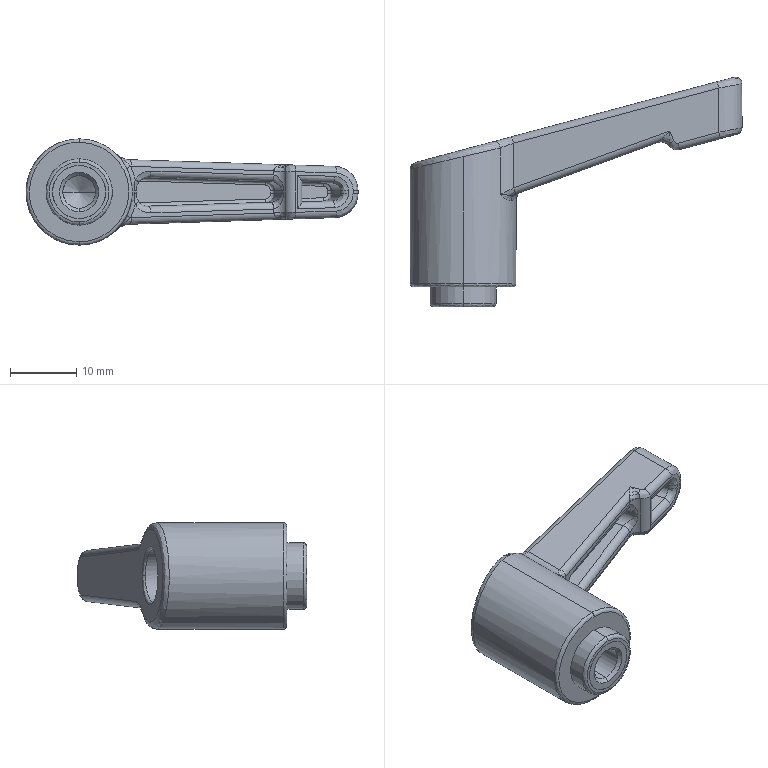Part | SolidWorks | features BaseBody 1 | 1 solid | 122 faces | box 50 x 34.597 x 16.002 mm | volume 5701 mm3 | cylinder 49 | spline 47 | plane 22 | cone 4 | commonest cylinder face diameters 2 x19 1 x8 2.8 x2 3 x2 4 x2 4.917 x2